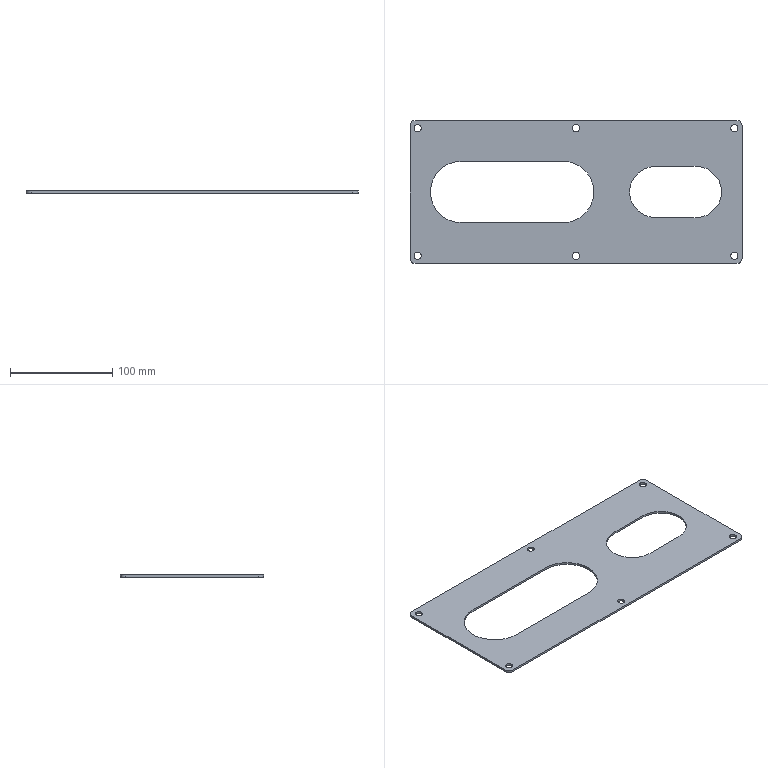Part | SolidWorks | features BaseBody 1 | 1 solid | 32 faces | box 325 x 140 x 2 mm | volume 64913 mm3 | cylinder 22 | plane 10 | commonest cylinder face diameters 7 x12 10 x4 50 x3 60 x3
STEP:
#1=CARTESIAN_POINT('',(-112.5,-30.,0.));
#2=VERTEX_POINT('',#1);
#3=CARTESIAN_POINT('',(-12.5,-30.,0.));
#4=VERTEX_POINT('',#3);
#5=CARTESIAN_POINT('',(-112.5,-30.,0.));
#6=DIRECTION('',(1.,0.,0.));
#7=VECTOR('',#6,1000.);
#8=LINE('',#5,#7);
#9=EDGE_CURVE('',#2,#4,#8,.T.);
#10=ORIENTED_EDGE('',*,*,#9,.T.);
#11=CARTESIAN_POINT('',(-12.5,-30.,-2.));
#12=VERTEX_POINT('',#11);
#13=CARTESIAN_POINT('',(-12.5,-30.,-2.));
#14=DIRECTION('',(0.,0.,1.));
#15=VECTOR('',#14,1000.);
#16=LINE('',#13,#15);
#17=EDGE_CURVE('',#12,#4,#16,.T.);
#18=ORIENTED_EDGE('',*,*,#17,.F.);
#19=CARTESIAN_POINT('',(-112.5,-30.,-2.));
#20=VERTEX_POINT('',#19);
#21=CARTESIAN_POINT('',(-112.5,-30.,-2.));
#22=DIRECTION('',(1.,0.,0.));
#23=VECTOR('',#22,1000.);
#24=LINE('',#21,#23);
#25=EDGE_CURVE('',#20,#12,#24,.T.);
#26=ORIENTED_EDGE('',*,*,#25,.F.);
#27=CARTESIAN_POINT('',(-112.5,-30.,-2.));
#28=DIRECTION('',(0.,0.,1.));
#29=VECTOR('',#28,1000.);
#30=LINE('',#27,#29);
#31=EDGE_CURVE('',#20,#2,#30,.T.);
#32=ORIENTED_EDGE('',*,*,#31,.T.);
#33=EDGE_LOOP('',(#10,#18,#26,#32));
#34=FACE_OUTER_BOUND('',#33,.T.);
#35=CARTESIAN_POINT('',(-112.5,-30.,-2.));
#36=DIRECTION('',(0.,-1.,0.));
#37=DIRECTION('',(-1.,0.,0.));
#38=AXIS2_PLACEMENT_3D('',#35,#36,#37);
#39=PLANE('',#38);
#40=ADVANCED_FACE('',(#34),#39,.F.);
#41=CARTESIAN_POINT('',(17.5,0.,-2.));
#42=VERTEX_POINT('',#41);
#43=CARTESIAN_POINT('',(17.5,0.,0.));
#44=VERTEX_POINT('',#43);
#45=CARTESIAN_POINT('',(17.5,0.,-2.));
#46=DIRECTION('',(0.,0.,1.));
#47=VECTOR('',#46,1000.);
#48=LINE('',#45,#47);
#49=EDGE_CURVE('',#42,#44,#48,.T.);
#50=ORIENTED_EDGE('',*,*,#49,.F.);
#51=CARTESIAN_POINT('',(-12.5,0.,-2.));
#52=DIRECTION('',(0.,0.,1.));
#53=DIRECTION('',(1.,0.,0.));
#54=AXIS2_PLACEMENT_3D('',#51,#52,#53);
#55=CIRCLE('',#54,30.);
#56=EDGE_CURVE('',#12,#42,#55,.T.);
#57=ORIENTED_EDGE('',*,*,#56,.F.);
#58=ORIENTED_EDGE('',*,*,#17,.T.);
#59=CARTESIAN_POINT('',(-12.5,0.,0.));
#60=DIRECTION('',(0.,0.,1.));
#61=DIRECTION('',(1.,0.,0.));
#62=AXIS2_PLACEMENT_3D('',#59,#60,#61);
#63=CIRCLE('',#62,30.);
#64=EDGE_CURVE('',#4,#44,#63,.T.);
#65=ORIENTED_EDGE('',*,*,#64,.T.);
#66=EDGE_LOOP('',(#50,#57,#58,#65));
#67=FACE_OUTER_BOUND('',#66,.T.);
#68=CARTESIAN_POINT('',(-12.5,0.,-2.));
#69=DIRECTION('',(0.,0.,1.));
#70=DIRECTION('',(1.,0.,0.));
#71=AXIS2_PLACEMENT_3D('',#68,#69,#70);
#72=CYLINDRICAL_SURFACE('',#71,30.);
#73=ADVANCED_FACE('',(#67),#72,.F.);
#74=CARTESIAN_POINT('',(-12.5,30.,0.));
#75=VERTEX_POINT('',#74);
#76=CARTESIAN_POINT('',(-112.5,30.,0.));
#77=VERTEX_POINT('',#76);
#78=CARTESIAN_POINT('',(-112.5,30.,0.));
#79=DIRECTION('',(-1.,0.,0.));
#80=VECTOR('',#79,1000.);
#81=LINE('',#78,#80);
#82=EDGE_CURVE('',#75,#77,#81,.T.);
#83=ORIENTED_EDGE('',*,*,#82,.T.);
#84=CARTESIAN_POINT('',(-112.5,30.,-2.));
#85=VERTEX_POINT('',#84);
#86=CARTESIAN_POINT('',(-112.5,30.,-2.));
#87=DIRECTION('',(0.,0.,1.));
#88=VECTOR('',#87,1000.);
#89=LINE('',#86,#88);
#90=EDGE_CURVE('',#85,#77,#89,.T.);
#91=ORIENTED_EDGE('',*,*,#90,.F.);
#92=CARTESIAN_POINT('',(-12.5,30.,-2.));
#93=VERTEX_POINT('',#92);
#94=CARTESIAN_POINT('',(-112.5,30.,-2.));
#95=DIRECTION('',(-1.,0.,0.));
#96=VECTOR('',#95,1000.);
#97=LINE('',#94,#96);
#98=EDGE_CURVE('',#93,#85,#97,.T.);
#99=ORIENTED_EDGE('',*,*,#98,.F.);
#100=CARTESIAN_POINT('',(-12.5,30.,-2.));
#101=DIRECTION('',(0.,0.,1.));
#102=VECTOR('',#101,1000.);
#103=LINE('',#100,#102);
#104=EDGE_CURVE('',#93,#75,#103,.T.);
#105=ORIENTED_EDGE('',*,*,#104,.T.);
#106=EDGE_LOOP('',(#83,#91,#99,#105));
#107=FACE_OUTER_BOUND('',#106,.T.);
#108=CARTESIAN_POINT('',(-112.5,30.,-2.));
#109=DIRECTION('',(0.,1.,0.));
#110=DIRECTION('',(1.,0.,0.));
#111=AXIS2_PLACEMENT_3D('',#108,#109,#110);
#112=PLANE('',#111);
#113=ADVANCED_FACE('',(#107),#112,.F.);
#114=CARTESIAN_POINT('',(-112.5,0.,0.));
#115=DIRECTION('',(0.,0.,1.));
#116=DIRECTION('',(1.,0.,0.));
#117=AXIS2_PLACEMENT_3D('',#114,#115,#116);
#118=CIRCLE('',#117,30.);
#119=EDGE_CURVE('',#77,#2,#118,.T.);
#120=ORIENTED_EDGE('',*,*,#119,.T.);
#121=ORIENTED_EDGE('',*,*,#31,.F.);
#122=CARTESIAN_POINT('',(-112.5,0.,-2.));
#123=DIRECTION('',(0.,0.,1.));
#124=DIRECTION('',(1.,0.,0.));
#125=AXIS2_PLACEMENT_3D('',#122,#123,#124);
#126=CIRCLE('',#125,30.);
#127=EDGE_CURVE('',#85,#20,#126,.T.);
#128=ORIENTED_EDGE('',*,*,#127,.F.);
#129=ORIENTED_EDGE('',*,*,#90,.T.);
#130=EDGE_LOOP('',(#120,#121,#128,#129));
#131=FACE_OUTER_BOUND('',#130,.T.);
#132=CARTESIAN_POINT('',(-112.5,0.,-2.));
#133=DIRECTION('',(0.,0.,1.));
#134=DIRECTION('',(1.,0.,0.));
#135=AXIS2_PLACEMENT_3D('',#132,#133,#134);
#136=CYLINDRICAL_SURFACE('',#135,30.);
#137=ADVANCED_FACE('',(#131),#136,.F.);
#138=CARTESIAN_POINT('',(77.5,-25.,0.));
#139=VERTEX_POINT('',#138);
#140=CARTESIAN_POINT('',(117.5,-25.,0.));
#141=VERTEX_POINT('',#140);
#142=CARTESIAN_POINT('',(77.5,-25.,0.));
#143=DIRECTION('',(1.,0.,0.));
#144=VECTOR('',#143,1000.);
#145=LINE('',#142,#144);
#146=EDGE_CURVE('',#139,#141,#145,.T.);
#147=ORIENTED_EDGE('',*,*,#146,.T.);
#148=CARTESIAN_POINT('',(117.5,-25.,-2.));
#149=VERTEX_POINT('',#148);
#150=CARTESIAN_POINT('',(117.5,-25.,-2.));
#151=DIRECTION('',(0.,0.,1.));
#152=VECTOR('',#151,1000.);
#153=LINE('',#150,#152);
#154=EDGE_CURVE('',#149,#141,#153,.T.);
#155=ORIENTED_EDGE('',*,*,#154,.F.);
#156=CARTESIAN_POINT('',(77.5,-25.,-2.));
#157=VERTEX_POINT('',#156);
#158=CARTESIAN_POINT('',(77.5,-25.,-2.));
#159=DIRECTION('',(1.,0.,0.));
#160=VECTOR('',#159,1000.);
#161=LINE('',#158,#160);
#162=EDGE_CURVE('',#157,#149,#161,.T.);
#163=ORIENTED_EDGE('',*,*,#162,.F.);
#164=CARTESIAN_POINT('',(77.5,-25.,-2.));
#165=DIRECTION('',(0.,0.,1.));
#166=VECTOR('',#165,1000.);
#167=LINE('',#164,#166);
#168=EDGE_CURVE('',#157,#139,#167,.T.);
#169=ORIENTED_EDGE('',*,*,#168,.T.);
#170=EDGE_LOOP('',(#147,#155,#163,#169));
#171=FACE_OUTER_BOUND('',#170,.T.);
#172=CARTESIAN_POINT('',(77.5,-25.,-2.));
#173=DIRECTION('',(0.,-1.,0.));
#174=DIRECTION('',(0.,0.,-1.));
#175=AXIS2_PLACEMENT_3D('',#172,#173,#174);
#176=PLANE('',#175);
#177=ADVANCED_FACE('',(#171),#176,.F.);
#178=CARTESIAN_POINT('',(142.5,0.,-2.));
#179=VERTEX_POINT('',#178);
#180=CARTESIAN_POINT('',(142.5,0.,0.));
#181=VERTEX_POINT('',#180);
#182=CARTESIAN_POINT('',(142.5,0.,-2.));
#183=DIRECTION('',(0.,0.,1.));
#184=VECTOR('',#183,1000.);
#185=LINE('',#182,#184);
#186=EDGE_CURVE('',#179,#181,#185,.T.);
#187=ORIENTED_EDGE('',*,*,#186,.F.);
#188=CARTESIAN_POINT('',(117.5,0.,-2.));
#189=DIRECTION('',(0.,0.,1.));
#190=DIRECTION('',(1.,0.,0.));
#191=AXIS2_PLACEMENT_3D('',#188,#189,#190);
#192=CIRCLE('',#191,25.);
#193=EDGE_CURVE('',#149,#179,#192,.T.);
#194=ORIENTED_EDGE('',*,*,#193,.F.);
#195=ORIENTED_EDGE('',*,*,#154,.T.);
#196=CARTESIAN_POINT('',(117.5,0.,0.));
#197=DIRECTION('',(0.,0.,1.));
#198=DIRECTION('',(1.,0.,0.));
#199=AXIS2_PLACEMENT_3D('',#196,#197,#198);
#200=CIRCLE('',#199,25.);
#201=EDGE_CURVE('',#141,#181,#200,.T.);
#202=ORIENTED_EDGE('',*,*,#201,.T.);
#203=EDGE_LOOP('',(#187,#194,#195,#202));
#204=FACE_OUTER_BOUND('',#203,.T.);
#205=CARTESIAN_POINT('',(117.5,0.,-2.));
#206=DIRECTION('',(0.,0.,1.));
#207=DIRECTION('',(1.,0.,0.));
#208=AXIS2_PLACEMENT_3D('',#205,#206,#207);
#209=CYLINDRICAL_SURFACE('',#208,25.);
#210=ADVANCED_FACE('',(#204),#209,.F.);
#211=CARTESIAN_POINT('',(117.5,25.,0.));
#212=VERTEX_POINT('',#211);
#213=CARTESIAN_POINT('',(77.5,25.,0.));
#214=VERTEX_POINT('',#213);
#215=CARTESIAN_POINT('',(77.5,25.,0.));
#216=DIRECTION('',(-1.,0.,0.));
#217=VECTOR('',#216,1000.);
#218=LINE('',#215,#217);
#219=EDGE_CURVE('',#212,#214,#218,.T.);
#220=ORIENTED_EDGE('',*,*,#219,.T.);
#221=CARTESIAN_POINT('',(77.5,25.,-2.));
#222=VERTEX_POINT('',#221);
#223=CARTESIAN_POINT('',(77.5,25.,-2.));
#224=DIRECTION('',(0.,0.,1.));
#225=VECTOR('',#224,1000.);
#226=LINE('',#223,#225);
#227=EDGE_CURVE('',#222,#214,#226,.T.);
#228=ORIENTED_EDGE('',*,*,#227,.F.);
#229=CARTESIAN_POINT('',(117.5,25.,-2.));
#230=VERTEX_POINT('',#229);
#231=CARTESIAN_POINT('',(77.5,25.,-2.));
#232=DIRECTION('',(-1.,0.,0.));
#233=VECTOR('',#232,1000.);
#234=LINE('',#231,#233);
#235=EDGE_CURVE('',#230,#222,#234,.T.);
#236=ORIENTED_EDGE('',*,*,#235,.F.);
#237=CARTESIAN_POINT('',(117.5,25.,-2.));
#238=DIRECTION('',(0.,0.,1.));
#239=VECTOR('',#238,1000.);
#240=LINE('',#237,#239);
#241=EDGE_CURVE('',#230,#212,#240,.T.);
#242=ORIENTED_EDGE('',*,*,#241,.T.);
#243=EDGE_LOOP('',(#220,#228,#236,#242));
#244=FACE_OUTER_BOUND('',#243,.T.);
#245=CARTESIAN_POINT('',(77.5,25.,-2.));
#246=DIRECTION('',(0.,1.,0.));
#247=DIRECTION('',(1.,0.,0.));
#248=AXIS2_PLACEMENT_3D('',#245,#246,#247);
#249=PLANE('',#248);
#250=ADVANCED_FACE('',(#244),#249,.F.);
#251=CARTESIAN_POINT('',(77.5,0.,0.));
#252=DIRECTION('',(0.,0.,1.));
#253=DIRECTION('',(1.,0.,0.));
#254=AXIS2_PLACEMENT_3D('',#251,#252,#253);
#255=CIRCLE('',#254,25.);
#256=EDGE_CURVE('',#214,#139,#255,.T.);
#257=ORIENTED_EDGE('',*,*,#256,.T.);
#258=ORIENTED_EDGE('',*,*,#168,.F.);
#259=CARTESIAN_POINT('',(77.5,0.,-2.));
#260=DIRECTION('',(0.,0.,1.));
#261=DIRECTION('',(1.,0.,0.));
#262=AXIS2_PLACEMENT_3D('',#259,#260,#261);
#263=CIRCLE('',#262,25.);
#264=EDGE_CURVE('',#222,#157,#263,.T.);
#265=ORIENTED_EDGE('',*,*,#264,.F.);
#266=ORIENTED_EDGE('',*,*,#227,.T.);
#267=EDGE_LOOP('',(#257,#258,#265,#266));
#268=FACE_OUTER_BOUND('',#267,.T.);
#269=CARTESIAN_POINT('',(77.5,0.,-2.));
#270=DIRECTION('',(0.,0.,1.));
#271=DIRECTION('',(1.,0.,0.));
#272=AXIS2_PLACEMENT_3D('',#269,#270,#271);
#273=CYLINDRICAL_SURFACE('',#272,25.);
#274=ADVANCED_FACE('',(#268),#273,.F.);
#275=CARTESIAN_POINT('',(-158.5,-62.5,-2.));
#276=VERTEX_POINT('',#275);
#277=CARTESIAN_POINT('',(-158.5,-62.5,0.));
#278=VERTEX_POINT('',#277);
#279=CARTESIAN_POINT('',(-158.5,-62.5,-2.));
#280=DIRECTION('',(0.,0.,1.));
#281=VECTOR('',#280,1000.);
#282=LINE('',#279,#281);
#283=EDGE_CURVE('',#276,#278,#282,.T.);
#284=ORIENTED_EDGE('',*,*,#283,.F.);
#285=CARTESIAN_POINT('',(-151.5,-62.5,-2.));
#286=VERTEX_POINT('',#285);
#287=CARTESIAN_POINT('',(-155.,-62.5,-2.));
#288=DIRECTION('',(0.,0.,1.));
#289=DIRECTION('',(-1.,0.,0.));
#290=AXIS2_PLACEMENT_3D('',#287,#288,#289);
#291=CIRCLE('',#290,3.5);
#292=EDGE_CURVE('',#286,#276,#291,.T.);
#293=ORIENTED_EDGE('',*,*,#292,.F.);
#294=CARTESIAN_POINT('',(-151.5,-62.5,0.));
#295=VERTEX_POINT('',#294);
#296=CARTESIAN_POINT('',(-151.5,-62.5,-2.));
#297=DIRECTION('',(0.,0.,1.));
#298=VECTOR('',#297,1000.);
#299=LINE('',#296,#298);
#300=EDGE_CURVE('',#286,#295,#299,.T.);
#301=ORIENTED_EDGE('',*,*,#300,.T.);
#302=CARTESIAN_POINT('',(-155.,-62.5,0.));
#303=DIRECTION('',(0.,0.,1.));
#304=DIRECTION('',(-1.,0.,0.));
#305=AXIS2_PLACEMENT_3D('',#302,#303,#304);
#306=CIRCLE('',#305,3.5);
#307=EDGE_CURVE('',#295,#278,#306,.T.);
#308=ORIENTED_EDGE('',*,*,#307,.T.);
#309=EDGE_LOOP('',(#284,#293,#301,#308));
#310=FACE_OUTER_BOUND('',#309,.T.);
#311=CARTESIAN_POINT('',(-155.,-62.5,-2.));
#312=DIRECTION('',(0.,0.,1.));
#313=DIRECTION('',(1.,0.,0.));
#314=AXIS2_PLACEMENT_3D('',#311,#312,#313);
#315=CYLINDRICAL_SURFACE('',#314,3.5);
#316=ADVANCED_FACE('',(#310),#315,.F.);
#317=CARTESIAN_POINT('',(-3.5,62.5,-2.));
#318=VERTEX_POINT('',#317);
#319=CARTESIAN_POINT('',(-3.5,62.5,0.));
#320=VERTEX_POINT('',#319);
#321=CARTESIAN_POINT('',(-3.5,62.5,-2.));
#322=DIRECTION('',(0.,0.,1.));
#323=VECTOR('',#322,1000.);
#324=LINE('',#321,#323);
#325=EDGE_CURVE('',#318,#320,#324,.T.);
#326=ORIENTED_EDGE('',*,*,#325,.F.);
#327=CARTESIAN_POINT('',(3.5,62.5,-2.));
#328=VERTEX_POINT('',#327);
#329=CARTESIAN_POINT('',(0.,62.5,-2.));
#330=DIRECTION('',(0.,0.,1.));
#331=DIRECTION('',(1.,0.,0.));
#332=AXIS2_PLACEMENT_3D('',#329,#330,#331);
#333=CIRCLE('',#332,3.5);
#334=EDGE_CURVE('',#328,#318,#333,.T.);
#335=ORIENTED_EDGE('',*,*,#334,.F.);
#336=CARTESIAN_POINT('',(3.5,62.5,0.));
#337=VERTEX_POINT('',#336);
#338=CARTESIAN_POINT('',(3.5,62.5,-2.));
#339=DIRECTION('',(0.,0.,1.));
#340=VECTOR('',#339,1000.);
#341=LINE('',#338,#340);
#342=EDGE_CURVE('',#328,#337,#341,.T.);
#343=ORIENTED_EDGE('',*,*,#342,.T.);
#344=CARTESIAN_POINT('',(0.,62.5,0.));
#345=DIRECTION('',(0.,0.,1.));
#346=DIRECTION('',(1.,0.,0.));
#347=AXIS2_PLACEMENT_3D('',#344,#345,#346);
#348=CIRCLE('',#347,3.5);
#349=EDGE_CURVE('',#337,#320,#348,.T.);
#350=ORIENTED_EDGE('',*,*,#349,.T.);
#351=EDGE_LOOP('',(#326,#335,#343,#350));
#352=FACE_OUTER_BOUND('',#351,.T.);
#353=CARTESIAN_POINT('',(0.,62.5,-2.));
#354=DIRECTION('',(0.,0.,1.));
#355=DIRECTION('',(1.,0.,0.));
#356=AXIS2_PLACEMENT_3D('',#353,#354,#355);
#357=CYLINDRICAL_SURFACE('',#356,3.5);
#358=ADVANCED_FACE('',(#352),#357,.F.);
#359=CARTESIAN_POINT('',(151.5,-62.5,-2.));
#360=VERTEX_POINT('',#359);
#361=CARTESIAN_POINT('',(151.5,-62.5,0.));
#362=VERTEX_POINT('',#361);
#363=CARTESIAN_POINT('',(151.5,-62.5,-2.));
#364=DIRECTION('',(0.,0.,1.));
#365=VECTOR('',#364,1000.);
#366=LINE('',#363,#365);
#367=EDGE_CURVE('',#360,#362,#366,.T.);
#368=ORIENTED_EDGE('',*,*,#367,.F.);
#369=CARTESIAN_POINT('',(158.5,-62.5,-2.));
#370=VERTEX_POINT('',#369);
#371=CARTESIAN_POINT('',(155.,-62.5,-2.));
#372=DIRECTION('',(0.,0.,1.));
#373=DIRECTION('',(1.,0.,0.));
#374=AXIS2_PLACEMENT_3D('',#371,#372,#373);
#375=CIRCLE('',#374,3.5);
#376=EDGE_CURVE('',#370,#360,#375,.T.);
#377=ORIENTED_EDGE('',*,*,#376,.F.);
#378=CARTESIAN_POINT('',(158.5,-62.5,0.));
#379=VERTEX_POINT('',#378);
#380=CARTESIAN_POINT('',(158.5,-62.5,-2.));
#381=DIRECTION('',(0.,0.,1.));
#382=VECTOR('',#381,1000.);
#383=LINE('',#380,#382);
#384=EDGE_CURVE('',#370,#379,#383,.T.);
#385=ORIENTED_EDGE('',*,*,#384,.T.);
#386=CARTESIAN_POINT('',(155.,-62.5,0.));
#387=DIRECTION('',(0.,0.,1.));
#388=DIRECTION('',(1.,0.,0.));
#389=AXIS2_PLACEMENT_3D('',#386,#387,#388);
#390=CIRCLE('',#389,3.5);
#391=EDGE_CURVE('',#379,#362,#390,.T.);
#392=ORIENTED_EDGE('',*,*,#391,.T.);
#393=EDGE_LOOP('',(#368,#377,#385,#392));
#394=FACE_OUTER_BOUND('',#393,.T.);
#395=CARTESIAN_POINT('',(155.,-62.5,-2.));
#396=DIRECTION('',(0.,0.,1.));
#397=DIRECTION('',(1.,0.,0.));
#398=AXIS2_PLACEMENT_3D('',#395,#396,#397);
#399=CYLINDRICAL_SURFACE('',#398,3.5);
#400=ADVANCED_FACE('',(#394),#399,.F.);
#401=CARTESIAN_POINT('',(151.5,62.5,-2.));
#402=VERTEX_POINT('',#401);
#403=CARTESIAN_POINT('',(151.5,62.5,0.));
#404=VERTEX_POINT('',#403);
#405=CARTESIAN_POINT('',(151.5,62.5,-2.));
#406=DIRECTION('',(0.,0.,1.));
#407=VECTOR('',#406,1000.);
#408=LINE('',#405,#407);
#409=EDGE_CURVE('',#402,#404,#408,.T.);
#410=ORIENTED_EDGE('',*,*,#409,.F.);
#411=CARTESIAN_POINT('',(158.5,62.5,-2.));
#412=VERTEX_POINT('',#411);
#413=CARTESIAN_POINT('',(155.,62.5,-2.));
#414=DIRECTION('',(0.,0.,1.));
#415=DIRECTION('',(-1.,0.,0.));
#416=AXIS2_PLACEMENT_3D('',#413,#414,#415);
#417=CIRCLE('',#416,3.5);
#418=EDGE_CURVE('',#412,#402,#417,.T.);
#419=ORIENTED_EDGE('',*,*,#418,.F.);
#420=CARTESIAN_POINT('',(158.5,62.5,0.));
#421=VERTEX_POINT('',#420);
#422=CARTESIAN_POINT('',(158.5,62.5,-2.));
#423=DIRECTION('',(0.,0.,1.));
#424=VECTOR('',#423,1000.);
#425=LINE('',#422,#424);
#426=EDGE_CURVE('',#412,#421,#425,.T.);
#427=ORIENTED_EDGE('',*,*,#426,.T.);
#428=CARTESIAN_POINT('',(155.,62.5,0.));
#429=DIRECTION('',(0.,0.,1.));
#430=DIRECTION('',(-1.,0.,0.));
#431=AXIS2_PLACEMENT_3D('',#428,#429,#430);
#432=CIRCLE('',#431,3.5);
#433=EDGE_CURVE('',#421,#404,#432,.T.);
#434=ORIENTED_EDGE('',*,*,#433,.T.);
#435=EDGE_LOOP('',(#410,#419,#427,#434));
#436=FACE_OUTER_BOUND('',#435,.T.);
#437=CARTESIAN_POINT('',(155.,62.5,-2.));
#438=DIRECTION('',(0.,0.,1.));
#439=DIRECTION('',(1.,0.,0.));
#440=AXIS2_PLACEMENT_3D('',#437,#438,#439);
#441=CYLINDRICAL_SURFACE('',#440,3.5);
#442=ADVANCED_FACE('',(#436),#441,.F.);
#443=CARTESIAN_POINT('',(-3.5,-62.5,-2.));
#444=VERTEX_POINT('',#443);
#445=CARTESIAN_POINT('',(-3.5,-62.5,0.));
#446=VERTEX_POINT('',#445);
#447=CARTESIAN_POINT('',(-3.5,-62.5,-2.));
#448=DIRECTION('',(0.,0.,1.));
#449=VECTOR('',#448,1000.);
#450=LINE('',#447,#449);
#451=EDGE_CURVE('',#444,#446,#450,.T.);
#452=ORIENTED_EDGE('',*,*,#451,.F.);
#453=CARTESIAN_POINT('',(3.5,-62.5,-2.));
#454=VERTEX_POINT('',#453);
#455=CARTESIAN_POINT('',(0.,-62.5,-2.));
#456=DIRECTION('',(0.,0.,1.));
#457=DIRECTION('',(-1.,0.,0.));
#458=AXIS2_PLACEMENT_3D('',#455,#456,#457);
#459=CIRCLE('',#458,3.5);
#460=EDGE_CURVE('',#454,#444,#459,.T.);
#461=ORIENTED_EDGE('',*,*,#460,.F.);
#462=CARTESIAN_POINT('',(3.5,-62.5,0.));
#463=VERTEX_POINT('',#462);
#464=CARTESIAN_POINT('',(3.5,-62.5,-2.));
#465=DIRECTION('',(0.,0.,1.));
#466=VECTOR('',#465,1000.);
#467=LINE('',#464,#466);
#468=EDGE_CURVE('',#454,#463,#467,.T.);
#469=ORIENTED_EDGE('',*,*,#468,.T.);
#470=CARTESIAN_POINT('',(0.,-62.5,0.));
#471=DIRECTION('',(0.,0.,1.));
#472=DIRECTION('',(-1.,0.,0.));
#473=AXIS2_PLACEMENT_3D('',#470,#471,#472);
#474=CIRCLE('',#473,3.5);
#475=EDGE_CURVE('',#463,#446,#474,.T.);
#476=ORIENTED_EDGE('',*,*,#475,.T.);
#477=EDGE_LOOP('',(#452,#461,#469,#476));
#478=FACE_OUTER_BOUND('',#477,.T.);
#479=CARTESIAN_POINT('',(0.,-62.5,-2.));
#480=DIRECTION('',(0.,0.,1.));
#481=DIRECTION('',(1.,0.,0.));
#482=AXIS2_PLACEMENT_3D('',#479,#480,#481);
#483=CYLINDRICAL_SURFACE('',#482,3.5);
#484=ADVANCED_FACE('',(#478),#483,.F.);
#485=CARTESIAN_POINT('',(-158.5,62.5,-2.));
#486=VERTEX_POINT('',#485);
#487=CARTESIAN_POINT('',(-158.5,62.5,0.));
#488=VERTEX_POINT('',#487);
#489=CARTESIAN_POINT('',(-158.5,62.5,-2.));
#490=DIRECTION('',(0.,0.,1.));
#491=VECTOR('',#490,1000.);
#492=LINE('',#489,#491);
#493=EDGE_CURVE('',#486,#488,#492,.T.);
#494=ORIENTED_EDGE('',*,*,#493,.F.);
#495=CARTESIAN_POINT('',(-151.5,62.5,-2.));
#496=VERTEX_POINT('',#495);
#497=CARTESIAN_POINT('',(-155.,62.5,-2.));
#498=DIRECTION('',(0.,0.,1.));
#499=DIRECTION('',(1.,0.,0.));
#500=AXIS2_PLACEMENT_3D('',#497,#498,#499);
#501=CIRCLE('',#500,3.5);
#502=EDGE_CURVE('',#496,#486,#501,.T.);
#503=ORIENTED_EDGE('',*,*,#502,.F.);
#504=CARTESIAN_POINT('',(-151.5,62.5,0.));
#505=VERTEX_POINT('',#504);
#506=CARTESIAN_POINT('',(-151.5,62.5,-2.));
#507=DIRECTION('',(0.,0.,1.));
#508=VECTOR('',#507,1000.);
#509=LINE('',#506,#508);
#510=EDGE_CURVE('',#496,#505,#509,.T.);
#511=ORIENTED_EDGE('',*,*,#510,.T.);
#512=CARTESIAN_POINT('',(-155.,62.5,0.));
#513=DIRECTION('',(0.,0.,1.));
#514=DIRECTION('',(1.,0.,0.));
#515=AXIS2_PLACEMENT_3D('',#512,#513,#514);
#516=CIRCLE('',#515,3.5);
#517=EDGE_CURVE('',#505,#488,#516,.T.);
#518=ORIENTED_EDGE('',*,*,#517,.T.);
#519=EDGE_LOOP('',(#494,#503,#511,#518));
#520=FACE_OUTER_BOUND('',#519,.T.);
#521=CARTESIAN_POINT('',(-155.,62.5,-2.));
#522=DIRECTION('',(0.,0.,1.));
#523=DIRECTION('',(1.,0.,0.));
#524=AXIS2_PLACEMENT_3D('',#521,#522,#523);
#525=CYLINDRICAL_SURFACE('',#524,3.5);
#526=ADVANCED_FACE('',(#520),#525,.F.);
#527=CARTESIAN_POINT('',(-162.5,65.,-2.));
#528=VERTEX_POINT('',#527);
#529=CARTESIAN_POINT('',(-157.5,70.,-2.));
#530=VERTEX_POINT('',#529);
#531=CARTESIAN_POINT('',(-157.5,65.,-2.));
#532=DIRECTION('',(0.,0.,-1.));
#533=DIRECTION('',(-1.,0.,0.));
#534=AXIS2_PLACEMENT_3D('',#531,#532,#533);
#535=CIRCLE('',#534,5.);
#536=EDGE_CURVE('',#528,#530,#535,.T.);
#537=ORIENTED_EDGE('',*,*,#536,.F.);
#538=CARTESIAN_POINT('',(-162.5,65.,0.));
#539=VERTEX_POINT('',#538);
#540=CARTESIAN_POINT('',(-162.5,65.,-2.));
#541=DIRECTION('',(0.,0.,-1.));
#542=VECTOR('',#541,1000.);
#543=LINE('',#540,#542);
#544=EDGE_CURVE('',#539,#528,#543,.T.);
#545=ORIENTED_EDGE('',*,*,#544,.F.);
#546=CARTESIAN_POINT('',(-157.5,70.,0.));
#547=VERTEX_POINT('',#546);
#548=CARTESIAN_POINT('',(-157.5,65.,0.));
#549=DIRECTION('',(0.,0.,1.));
#550=DIRECTION('',(-1.,0.,0.));
#551=AXIS2_PLACEMENT_3D('',#548,#549,#550);
#552=CIRCLE('',#551,5.);
#553=EDGE_CURVE('',#547,#539,#552,.T.);
#554=ORIENTED_EDGE('',*,*,#553,.F.);
#555=CARTESIAN_POINT('',(-157.5,70.,-2.));
#556=DIRECTION('',(0.,0.,1.));
#557=VECTOR('',#556,1000.);
#558=LINE('',#555,#557);
#559=EDGE_CURVE('',#530,#547,#558,.T.);
#560=ORIENTED_EDGE('',*,*,#559,.F.);
#561=EDGE_LOOP('',(#537,#545,#554,#560));
#562=FACE_OUTER_BOUND('',#561,.T.);
#563=CARTESIAN_POINT('',(-157.5,65.,-2.));
#564=DIRECTION('',(0.,0.,1.));
#565=DIRECTION('',(1.,0.,0.));
#566=AXIS2_PLACEMENT_3D('',#563,#564,#565);
#567=CYLINDRICAL_SURFACE('',#566,5.);
#568=ADVANCED_FACE('',(#562),#567,.T.);
#569=CARTESIAN_POINT('',(-157.5,-70.,-2.));
#570=VERTEX_POINT('',#569);
#571=CARTESIAN_POINT('',(-162.5,-65.,-2.));
#572=VERTEX_POINT('',#571);
#573=CARTESIAN_POINT('',(-157.5,-65.,-2.));
#574=DIRECTION('',(0.,0.,-1.));
#575=DIRECTION('',(-1.,0.,0.));
#576=AXIS2_PLACEMENT_3D('',#573,#574,#575);
#577=CIRCLE('',#576,5.);
#578=EDGE_CURVE('',#570,#572,#577,.T.);
#579=ORIENTED_EDGE('',*,*,#578,.F.);
#580=CARTESIAN_POINT('',(-157.5,-70.,0.));
#581=VERTEX_POINT('',#580);
#582=CARTESIAN_POINT('',(-157.5,-70.,-2.));
#583=DIRECTION('',(0.,0.,-1.));
#584=VECTOR('',#583,1000.);
#585=LINE('',#582,#584);
#586=EDGE_CURVE('',#581,#570,#585,.T.);
#587=ORIENTED_EDGE('',*,*,#586,.F.);
#588=CARTESIAN_POINT('',(-162.5,-65.,0.));
#589=VERTEX_POINT('',#588);
#590=CARTESIAN_POINT('',(-157.5,-65.,0.));
#591=DIRECTION('',(0.,0.,1.));
#592=DIRECTION('',(-1.,0.,0.));
#593=AXIS2_PLACEMENT_3D('',#590,#591,#592);
#594=CIRCLE('',#593,5.);
#595=EDGE_CURVE('',#589,#581,#594,.T.);
#596=ORIENTED_EDGE('',*,*,#595,.F.);
#597=CARTESIAN_POINT('',(-162.5,-65.,-2.));
#598=DIRECTION('',(0.,0.,1.));
#599=VECTOR('',#598,1000.);
#600=LINE('',#597,#599);
#601=EDGE_CURVE('',#572,#589,#600,.T.);
#602=ORIENTED_EDGE('',*,*,#601,.F.);
#603=EDGE_LOOP('',(#579,#587,#596,#602));
#604=FACE_OUTER_BOUND('',#603,.T.);
#605=CARTESIAN_POINT('',(-157.5,-65.,-2.));
#606=DIRECTION('',(0.,0.,1.));
#607=DIRECTION('',(1.,0.,0.));
#608=AXIS2_PLACEMENT_3D('',#605,#606,#607);
#609=CYLINDRICAL_SURFACE('',#608,5.);
#610=ADVANCED_FACE('',(#604),#609,.T.);
#611=CARTESIAN_POINT('',(162.5,-65.,-2.));
#612=VERTEX_POINT('',#611);
#613=CARTESIAN_POINT('',(157.5,-70.,-2.));
#614=VERTEX_POINT('',#613);
#615=CARTESIAN_POINT('',(157.5,-65.,-2.));
#616=DIRECTION('',(0.,0.,-1.));
#617=DIRECTION('',(-1.,0.,0.));
#618=AXIS2_PLACEMENT_3D('',#615,#616,#617);
#619=CIRCLE('',#618,5.);
#620=EDGE_CURVE('',#612,#614,#619,.T.);
#621=ORIENTED_EDGE('',*,*,#620,.F.);
#622=CARTESIAN_POINT('',(162.5,-65.,0.));
#623=VERTEX_POINT('',#622);
#624=CARTESIAN_POINT('',(162.5,-65.,-2.));
#625=DIRECTION('',(0.,0.,-1.));
#626=VECTOR('',#625,1000.);
#627=LINE('',#624,#626);
#628=EDGE_CURVE('',#623,#612,#627,.T.);
#629=ORIENTED_EDGE('',*,*,#628,.F.);
#630=CARTESIAN_POINT('',(157.5,-70.,0.));
#631=VERTEX_POINT('',#630);
#632=CARTESIAN_POINT('',(157.5,-65.,0.));
#633=DIRECTION('',(0.,0.,1.));
#634=DIRECTION('',(-1.,0.,0.));
#635=AXIS2_PLACEMENT_3D('',#632,#633,#634);
#636=CIRCLE('',#635,5.);
#637=EDGE_CURVE('',#631,#623,#636,.T.);
#638=ORIENTED_EDGE('',*,*,#637,.F.);
#639=CARTESIAN_POINT('',(157.5,-70.,-2.));
#640=DIRECTION('',(0.,0.,1.));
#641=VECTOR('',#640,1000.);
#642=LINE('',#639,#641);
#643=EDGE_CURVE('',#614,#631,#642,.T.);
#644=ORIENTED_EDGE('',*,*,#643,.F.);
#645=EDGE_LOOP('',(#621,#629,#638,#644));
#646=FACE_OUTER_BOUND('',#645,.T.);
#647=CARTESIAN_POINT('',(157.5,-65.,-2.));
#648=DIRECTION('',(0.,0.,1.));
#649=DIRECTION('',(1.,0.,0.));
#650=AXIS2_PLACEMENT_3D('',#647,#648,#649);
#651=CYLINDRICAL_SURFACE('',#650,5.);
#652=ADVANCED_FACE('',(#646),#651,.T.);
#653=CARTESIAN_POINT('',(157.5,70.,-2.));
#654=VERTEX_POINT('',#653);
#655=CARTESIAN_POINT('',(162.5,65.,-2.));
#656=VERTEX_POINT('',#655);
#657=CARTESIAN_POINT('',(157.5,65.,-2.));
#658=DIRECTION('',(0.,0.,-1.));
#659=DIRECTION('',(-1.,0.,0.));
#660=AXIS2_PLACEMENT_3D('',#657,#658,#659);
#661=CIRCLE('',#660,5.);
#662=EDGE_CURVE('',#654,#656,#661,.T.);
#663=ORIENTED_EDGE('',*,*,#662,.F.);
#664=CARTESIAN_POINT('',(157.5,70.,0.));
#665=VERTEX_POINT('',#664);
#666=CARTESIAN_POINT('',(157.5,70.,-2.));
#667=DIRECTION('',(0.,0.,-1.));
#668=VECTOR('',#667,1000.);
#669=LINE('',#666,#668);
#670=EDGE_CURVE('',#665,#654,#669,.T.);
#671=ORIENTED_EDGE('',*,*,#670,.F.);
#672=CARTESIAN_POINT('',(162.5,65.,0.));
#673=VERTEX_POINT('',#672);
#674=CARTESIAN_POINT('',(157.5,65.,0.));
#675=DIRECTION('',(0.,0.,1.));
#676=DIRECTION('',(-1.,0.,0.));
#677=AXIS2_PLACEMENT_3D('',#674,#675,#676);
#678=CIRCLE('',#677,5.);
#679=EDGE_CURVE('',#673,#665,#678,.T.);
#680=ORIENTED_EDGE('',*,*,#679,.F.);
#681=CARTESIAN_POINT('',(162.5,65.,-2.));
#682=DIRECTION('',(0.,0.,1.));
#683=VECTOR('',#682,1000.);
#684=LINE('',#681,#683);
#685=EDGE_CURVE('',#656,#673,#684,.T.);
#686=ORIENTED_EDGE('',*,*,#685,.F.);
#687=EDGE_LOOP('',(#663,#671,#680,#686));
#688=FACE_OUTER_BOUND('',#687,.T.);
#689=CARTESIAN_POINT('',(157.5,65.,-2.));
#690=DIRECTION('',(0.,0.,1.));
#691=DIRECTION('',(1.,0.,0.));
#692=AXIS2_PLACEMENT_3D('',#689,#690,#691);
#693=CYLINDRICAL_SURFACE('',#692,5.);
#694=ADVANCED_FACE('',(#688),#693,.T.);
#695=ORIENTED_EDGE('',*,*,#517,.F.);
#696=CARTESIAN_POINT('',(-155.,62.5,0.));
#697=DIRECTION('',(0.,0.,1.));
#698=DIRECTION('',(1.,0.,0.));
#699=AXIS2_PLACEMENT_3D('',#696,#697,#698);
#700=CIRCLE('',#699,3.5);
#701=EDGE_CURVE('',#488,#505,#700,.T.);
#702=ORIENTED_EDGE('',*,*,#701,.F.);
#703=EDGE_LOOP('',(#695,#702));
#704=FACE_BOUND('',#703,.T.);
#705=ORIENTED_EDGE('',*,*,#475,.F.);
#706=CARTESIAN_POINT('',(0.,-62.5,0.));
#707=DIRECTION('',(0.,0.,1.));
#708=DIRECTION('',(-1.,0.,0.));
#709=AXIS2_PLACEMENT_3D('',#706,#707,#708);
#710=CIRCLE('',#709,3.5);
#711=EDGE_CURVE('',#446,#463,#710,.T.);
#712=ORIENTED_EDGE('',*,*,#711,.F.);
#713=EDGE_LOOP('',(#705,#712));
#714=FACE_BOUND('',#713,.T.);
#715=ORIENTED_EDGE('',*,*,#433,.F.);
#716=CARTESIAN_POINT('',(155.,62.5,0.));
#717=DIRECTION('',(0.,0.,1.));
#718=DIRECTION('',(-1.,0.,0.));
#719=AXIS2_PLACEMENT_3D('',#716,#717,#718);
#720=CIRCLE('',#719,3.5);
#721=EDGE_CURVE('',#404,#421,#720,.T.);
#722=ORIENTED_EDGE('',*,*,#721,.F.);
#723=EDGE_LOOP('',(#715,#722));
#724=FACE_BOUND('',#723,.T.);
#725=ORIENTED_EDGE('',*,*,#391,.F.);
#726=CARTESIAN_POINT('',(155.,-62.5,0.));
#727=DIRECTION('',(0.,0.,1.));
#728=DIRECTION('',(1.,0.,0.));
#729=AXIS2_PLACEMENT_3D('',#726,#727,#728);
#730=CIRCLE('',#729,3.5);
#731=EDGE_CURVE('',#362,#379,#730,.T.);
#732=ORIENTED_EDGE('',*,*,#731,.F.);
#733=EDGE_LOOP('',(#725,#732));
#734=FACE_BOUND('',#733,.T.);
#735=ORIENTED_EDGE('',*,*,#349,.F.);
#736=CARTESIAN_POINT('',(0.,62.5,0.));
#737=DIRECTION('',(0.,0.,1.));
#738=DIRECTION('',(1.,0.,0.));
#739=AXIS2_PLACEMENT_3D('',#736,#737,#738);
#740=CIRCLE('',#739,3.5);
#741=EDGE_CURVE('',#320,#337,#740,.T.);
#742=ORIENTED_EDGE('',*,*,#741,.F.);
#743=EDGE_LOOP('',(#735,#742));
#744=FACE_BOUND('',#743,.T.);
#745=ORIENTED_EDGE('',*,*,#307,.F.);
#746=CARTESIAN_POINT('',(-155.,-62.5,0.));
#747=DIRECTION('',(0.,0.,1.));
#748=DIRECTION('',(-1.,0.,0.));
#749=AXIS2_PLACEMENT_3D('',#746,#747,#748);
#750=CIRCLE('',#749,3.5);
#751=EDGE_CURVE('',#278,#295,#750,.T.);
#752=ORIENTED_EDGE('',*,*,#751,.F.);
#753=EDGE_LOOP('',(#745,#752));
#754=FACE_BOUND('',#753,.T.);
#755=ORIENTED_EDGE('',*,*,#146,.F.);
#756=ORIENTED_EDGE('',*,*,#256,.F.);
#757=ORIENTED_EDGE('',*,*,#219,.F.);
#758=CARTESIAN_POINT('',(117.5,0.,0.));
#759=DIRECTION('',(0.,0.,1.));
#760=DIRECTION('',(1.,0.,0.));
#761=AXIS2_PLACEMENT_3D('',#758,#759,#760);
#762=CIRCLE('',#761,25.);
#763=EDGE_CURVE('',#181,#212,#762,.T.);
#764=ORIENTED_EDGE('',*,*,#763,.F.);
#765=ORIENTED_EDGE('',*,*,#201,.F.);
#766=EDGE_LOOP('',(#755,#756,#757,#764,#765));
#767=FACE_BOUND('',#766,.T.);
#768=ORIENTED_EDGE('',*,*,#9,.F.);
#769=ORIENTED_EDGE('',*,*,#119,.F.);
#770=ORIENTED_EDGE('',*,*,#82,.F.);
#771=CARTESIAN_POINT('',(-12.5,0.,0.));
#772=DIRECTION('',(0.,0.,1.));
#773=DIRECTION('',(1.,0.,0.));
#774=AXIS2_PLACEMENT_3D('',#771,#772,#773);
#775=CIRCLE('',#774,30.);
#776=EDGE_CURVE('',#44,#75,#775,.T.);
#777=ORIENTED_EDGE('',*,*,#776,.F.);
#778=ORIENTED_EDGE('',*,*,#64,.F.);
#779=EDGE_LOOP('',(#768,#769,#770,#777,#778));
#780=FACE_BOUND('',#779,.T.);
#781=CARTESIAN_POINT('',(162.5,70.,0.));
#782=DIRECTION('',(0.,1.,0.));
#783=VECTOR('',#782,1000.);
#784=LINE('',#781,#783);
#785=EDGE_CURVE('',#623,#673,#784,.T.);
#786=ORIENTED_EDGE('',*,*,#785,.T.);
#787=ORIENTED_EDGE('',*,*,#679,.T.);
#788=CARTESIAN_POINT('',(162.5,70.,0.));
#789=DIRECTION('',(-1.,0.,0.));
#790=VECTOR('',#789,1000.);
#791=LINE('',#788,#790);
#792=EDGE_CURVE('',#665,#547,#791,.T.);
#793=ORIENTED_EDGE('',*,*,#792,.T.);
#794=ORIENTED_EDGE('',*,*,#553,.T.);
#795=CARTESIAN_POINT('',(-162.5,70.,0.));
#796=DIRECTION('',(0.,-1.,0.));
#797=VECTOR('',#796,1000.);
#798=LINE('',#795,#797);
#799=EDGE_CURVE('',#539,#589,#798,.T.);
#800=ORIENTED_EDGE('',*,*,#799,.T.);
#801=ORIENTED_EDGE('',*,*,#595,.T.);
#802=CARTESIAN_POINT('',(162.5,-70.,0.));
#803=DIRECTION('',(1.,0.,0.));
#804=VECTOR('',#803,1000.);
#805=LINE('',#802,#804);
#806=EDGE_CURVE('',#581,#631,#805,.T.);
#807=ORIENTED_EDGE('',*,*,#806,.T.);
#808=ORIENTED_EDGE('',*,*,#637,.T.);
#809=EDGE_LOOP('',(#786,#787,#793,#794,#800,#801,#807,#808));
#810=FACE_OUTER_BOUND('',#809,.T.);
#811=CARTESIAN_POINT('',(0.,0.,0.));
#812=DIRECTION('',(0.,0.,-1.));
#813=DIRECTION('',(0.,-1.,0.));
#814=AXIS2_PLACEMENT_3D('',#811,#812,#813);
#815=PLANE('',#814);
#816=ADVANCED_FACE('',(#704,#714,#724,#734,#744,#754,#767,#780,#810),#815,.F.);
#817=ORIENTED_EDGE('',*,*,#502,.T.);
#818=CARTESIAN_POINT('',(-155.,62.5,-2.));
#819=DIRECTION('',(0.,0.,1.));
#820=DIRECTION('',(1.,0.,0.));
#821=AXIS2_PLACEMENT_3D('',#818,#819,#820);
#822=CIRCLE('',#821,3.5);
#823=EDGE_CURVE('',#486,#496,#822,.T.);
#824=ORIENTED_EDGE('',*,*,#823,.T.);
#825=EDGE_LOOP('',(#817,#824));
#826=FACE_BOUND('',#825,.T.);
#827=ORIENTED_EDGE('',*,*,#460,.T.);
#828=CARTESIAN_POINT('',(0.,-62.5,-2.));
#829=DIRECTION('',(0.,0.,1.));
#830=DIRECTION('',(-1.,0.,0.));
#831=AXIS2_PLACEMENT_3D('',#828,#829,#830);
#832=CIRCLE('',#831,3.5);
#833=EDGE_CURVE('',#444,#454,#832,.T.);
#834=ORIENTED_EDGE('',*,*,#833,.T.);
#835=EDGE_LOOP('',(#827,#834));
#836=FACE_BOUND('',#835,.T.);
#837=ORIENTED_EDGE('',*,*,#418,.T.);
#838=CARTESIAN_POINT('',(155.,62.5,-2.));
#839=DIRECTION('',(0.,0.,1.));
#840=DIRECTION('',(-1.,0.,0.));
#841=AXIS2_PLACEMENT_3D('',#838,#839,#840);
#842=CIRCLE('',#841,3.5);
#843=EDGE_CURVE('',#402,#412,#842,.T.);
#844=ORIENTED_EDGE('',*,*,#843,.T.);
#845=EDGE_LOOP('',(#837,#844));
#846=FACE_BOUND('',#845,.T.);
#847=ORIENTED_EDGE('',*,*,#376,.T.);
#848=CARTESIAN_POINT('',(155.,-62.5,-2.));
#849=DIRECTION('',(0.,0.,1.));
#850=DIRECTION('',(1.,0.,0.));
#851=AXIS2_PLACEMENT_3D('',#848,#849,#850);
#852=CIRCLE('',#851,3.5);
#853=EDGE_CURVE('',#360,#370,#852,.T.);
#854=ORIENTED_EDGE('',*,*,#853,.T.);
#855=EDGE_LOOP('',(#847,#854));
#856=FACE_BOUND('',#855,.T.);
#857=ORIENTED_EDGE('',*,*,#334,.T.);
#858=CARTESIAN_POINT('',(0.,62.5,-2.));
#859=DIRECTION('',(0.,0.,1.));
#860=DIRECTION('',(1.,0.,0.));
#861=AXIS2_PLACEMENT_3D('',#858,#859,#860);
#862=CIRCLE('',#861,3.5);
#863=EDGE_CURVE('',#318,#328,#862,.T.);
#864=ORIENTED_EDGE('',*,*,#863,.T.);
#865=EDGE_LOOP('',(#857,#864));
#866=FACE_BOUND('',#865,.T.);
#867=ORIENTED_EDGE('',*,*,#292,.T.);
#868=CARTESIAN_POINT('',(-155.,-62.5,-2.));
#869=DIRECTION('',(0.,0.,1.));
#870=DIRECTION('',(-1.,0.,0.));
#871=AXIS2_PLACEMENT_3D('',#868,#869,#870);
#872=CIRCLE('',#871,3.5);
#873=EDGE_CURVE('',#276,#286,#872,.T.);
#874=ORIENTED_EDGE('',*,*,#873,.T.);
#875=EDGE_LOOP('',(#867,#874));
#876=FACE_BOUND('',#875,.T.);
#877=ORIENTED_EDGE('',*,*,#264,.T.);
#878=ORIENTED_EDGE('',*,*,#162,.T.);
#879=ORIENTED_EDGE('',*,*,#193,.T.);
#880=CARTESIAN_POINT('',(117.5,0.,-2.));
#881=DIRECTION('',(0.,0.,1.));
#882=DIRECTION('',(1.,0.,0.));
#883=AXIS2_PLACEMENT_3D('',#880,#881,#882);
#884=CIRCLE('',#883,25.);
#885=EDGE_CURVE('',#179,#230,#884,.T.);
#886=ORIENTED_EDGE('',*,*,#885,.T.);
#887=ORIENTED_EDGE('',*,*,#235,.T.);
#888=EDGE_LOOP('',(#877,#878,#879,#886,#887));
#889=FACE_BOUND('',#888,.T.);
#890=ORIENTED_EDGE('',*,*,#127,.T.);
#891=ORIENTED_EDGE('',*,*,#25,.T.);
#892=ORIENTED_EDGE('',*,*,#56,.T.);
#893=CARTESIAN_POINT('',(-12.5,0.,-2.));
#894=DIRECTION('',(0.,0.,1.));
#895=DIRECTION('',(1.,0.,0.));
#896=AXIS2_PLACEMENT_3D('',#893,#894,#895);
#897=CIRCLE('',#896,30.);
#898=EDGE_CURVE('',#42,#93,#897,.T.);
#899=ORIENTED_EDGE('',*,*,#898,.T.);
#900=ORIENTED_EDGE('',*,*,#98,.T.);
#901=EDGE_LOOP('',(#890,#891,#892,#899,#900));
#902=FACE_BOUND('',#901,.T.);
#903=CARTESIAN_POINT('',(162.5,70.,-2.));
#904=DIRECTION('',(-1.,0.,0.));
#905=VECTOR('',#904,1000.);
#906=LINE('',#903,#905);
#907=EDGE_CURVE('',#654,#530,#906,.T.);
#908=ORIENTED_EDGE('',*,*,#907,.F.);
#909=ORIENTED_EDGE('',*,*,#662,.T.);
#910=CARTESIAN_POINT('',(162.5,70.,-2.));
#911=DIRECTION('',(0.,1.,0.));
#912=VECTOR('',#911,1000.);
#913=LINE('',#910,#912);
#914=EDGE_CURVE('',#612,#656,#913,.T.);
#915=ORIENTED_EDGE('',*,*,#914,.F.);
#916=ORIENTED_EDGE('',*,*,#620,.T.);
#917=CARTESIAN_POINT('',(162.5,-70.,-2.));
#918=DIRECTION('',(1.,0.,0.));
#919=VECTOR('',#918,1000.);
#920=LINE('',#917,#919);
#921=EDGE_CURVE('',#570,#614,#920,.T.);
#922=ORIENTED_EDGE('',*,*,#921,.F.);
#923=ORIENTED_EDGE('',*,*,#578,.T.);
#924=CARTESIAN_POINT('',(-162.5,70.,-2.));
#925=DIRECTION('',(0.,-1.,0.));
#926=VECTOR('',#925,1000.);
#927=LINE('',#924,#926);
#928=EDGE_CURVE('',#528,#572,#927,.T.);
#929=ORIENTED_EDGE('',*,*,#928,.F.);
#930=ORIENTED_EDGE('',*,*,#536,.T.);
#931=EDGE_LOOP('',(#908,#909,#915,#916,#922,#923,#929,#930));
#932=FACE_OUTER_BOUND('',#931,.T.);
#933=CARTESIAN_POINT('',(0.,0.,-2.));
#934=DIRECTION('',(0.,0.,-1.));
#935=DIRECTION('',(0.,-1.,0.));
#936=AXIS2_PLACEMENT_3D('',#933,#934,#935);
#937=PLANE('',#936);
#938=ADVANCED_FACE('',(#826,#836,#846,#856,#866,#876,#889,#902,#932),#937,.T.);
#939=ORIENTED_EDGE('',*,*,#921,.T.);
#940=ORIENTED_EDGE('',*,*,#643,.T.);
#941=ORIENTED_EDGE('',*,*,#806,.F.);
#942=ORIENTED_EDGE('',*,*,#586,.T.);
#943=EDGE_LOOP('',(#939,#940,#941,#942));
#944=FACE_OUTER_BOUND('',#943,.T.);
#945=CARTESIAN_POINT('',(162.5,-70.,-2.));
#946=DIRECTION('',(0.,-1.,0.));
#947=DIRECTION('',(0.,0.,-1.));
#948=AXIS2_PLACEMENT_3D('',#945,#946,#947);
#949=PLANE('',#948);
#950=ADVANCED_FACE('',(#944),#949,.T.);
#951=ORIENTED_EDGE('',*,*,#914,.T.);
#952=ORIENTED_EDGE('',*,*,#685,.T.);
#953=ORIENTED_EDGE('',*,*,#785,.F.);
#954=ORIENTED_EDGE('',*,*,#628,.T.);
#955=EDGE_LOOP('',(#951,#952,#953,#954));
#956=FACE_OUTER_BOUND('',#955,.T.);
#957=CARTESIAN_POINT('',(162.5,70.,-2.));
#958=DIRECTION('',(1.,0.,0.));
#959=DIRECTION('',(0.,1.,0.));
#960=AXIS2_PLACEMENT_3D('',#957,#958,#959);
#961=PLANE('',#960);
#962=ADVANCED_FACE('',(#956),#961,.T.);
#963=ORIENTED_EDGE('',*,*,#792,.F.);
#964=ORIENTED_EDGE('',*,*,#670,.T.);
#965=ORIENTED_EDGE('',*,*,#907,.T.);
#966=ORIENTED_EDGE('',*,*,#559,.T.);
#967=EDGE_LOOP('',(#963,#964,#965,#966));
#968=FACE_OUTER_BOUND('',#967,.T.);
#969=CARTESIAN_POINT('',(162.5,70.,-2.));
#970=DIRECTION('',(0.,1.,0.));
#971=DIRECTION('',(1.,0.,0.));
#972=AXIS2_PLACEMENT_3D('',#969,#970,#971);
#973=PLANE('',#972);
#974=ADVANCED_FACE('',(#968),#973,.T.);
#975=ORIENTED_EDGE('',*,*,#928,.T.);
#976=ORIENTED_EDGE('',*,*,#601,.T.);
#977=ORIENTED_EDGE('',*,*,#799,.F.);
#978=ORIENTED_EDGE('',*,*,#544,.T.);
#979=EDGE_LOOP('',(#975,#976,#977,#978));
#980=FACE_OUTER_BOUND('',#979,.T.);
#981=CARTESIAN_POINT('',(-162.5,70.,-2.));
#982=DIRECTION('',(-1.,0.,0.));
#983=DIRECTION('',(0.,1.,0.));
#984=AXIS2_PLACEMENT_3D('',#981,#982,#983);
#985=PLANE('',#984);
#986=ADVANCED_FACE('',(#980),#985,.T.);
#987=ORIENTED_EDGE('',*,*,#823,.F.);
#988=ORIENTED_EDGE('',*,*,#493,.T.);
#989=ORIENTED_EDGE('',*,*,#701,.T.);
#990=ORIENTED_EDGE('',*,*,#510,.F.);
#991=EDGE_LOOP('',(#987,#988,#989,#990));
#992=FACE_OUTER_BOUND('',#991,.T.);
#993=CARTESIAN_POINT('',(-155.,62.5,-2.));
#994=DIRECTION('',(0.,0.,1.));
#995=DIRECTION('',(1.,0.,0.));
#996=AXIS2_PLACEMENT_3D('',#993,#994,#995);
#997=CYLINDRICAL_SURFACE('',#996,3.5);
#998=ADVANCED_FACE('',(#992),#997,.F.);
#999=ORIENTED_EDGE('',*,*,#833,.F.);
#1000=ORIENTED_EDGE('',*,*,#451,.T.);
#1001=ORIENTED_EDGE('',*,*,#711,.T.);
#1002=ORIENTED_EDGE('',*,*,#468,.F.);
#1003=EDGE_LOOP('',(#999,#1000,#1001,#1002));
#1004=FACE_OUTER_BOUND('',#1003,.T.);
#1005=CARTESIAN_POINT('',(0.,-62.5,-2.));
#1006=DIRECTION('',(0.,0.,1.));
#1007=DIRECTION('',(1.,0.,0.));
#1008=AXIS2_PLACEMENT_3D('',#1005,#1006,#1007);
#1009=CYLINDRICAL_SURFACE('',#1008,3.5);
#1010=ADVANCED_FACE('',(#1004),#1009,.F.);
#1011=ORIENTED_EDGE('',*,*,#843,.F.);
#1012=ORIENTED_EDGE('',*,*,#409,.T.);
#1013=ORIENTED_EDGE('',*,*,#721,.T.);
#1014=ORIENTED_EDGE('',*,*,#426,.F.);
#1015=EDGE_LOOP('',(#1011,#1012,#1013,#1014));
#1016=FACE_OUTER_BOUND('',#1015,.T.);
#1017=CARTESIAN_POINT('',(155.,62.5,-2.));
#1018=DIRECTION('',(0.,0.,1.));
#1019=DIRECTION('',(1.,0.,0.));
#1020=AXIS2_PLACEMENT_3D('',#1017,#1018,#1019);
#1021=CYLINDRICAL_SURFACE('',#1020,3.5);
#1022=ADVANCED_FACE('',(#1016),#1021,.F.);
#1023=ORIENTED_EDGE('',*,*,#853,.F.);
#1024=ORIENTED_EDGE('',*,*,#367,.T.);
#1025=ORIENTED_EDGE('',*,*,#731,.T.);
#1026=ORIENTED_EDGE('',*,*,#384,.F.);
#1027=EDGE_LOOP('',(#1023,#1024,#1025,#1026));
#1028=FACE_OUTER_BOUND('',#1027,.T.);
#1029=CARTESIAN_POINT('',(155.,-62.5,-2.));
#1030=DIRECTION('',(0.,0.,1.));
#1031=DIRECTION('',(1.,0.,0.));
#1032=AXIS2_PLACEMENT_3D('',#1029,#1030,#1031);
#1033=CYLINDRICAL_SURFACE('',#1032,3.5);
#1034=ADVANCED_FACE('',(#1028),#1033,.F.);
#1035=ORIENTED_EDGE('',*,*,#863,.F.);
#1036=ORIENTED_EDGE('',*,*,#325,.T.);
#1037=ORIENTED_EDGE('',*,*,#741,.T.);
#1038=ORIENTED_EDGE('',*,*,#342,.F.);
#1039=EDGE_LOOP('',(#1035,#1036,#1037,#1038));
#1040=FACE_OUTER_BOUND('',#1039,.T.);
#1041=CARTESIAN_POINT('',(0.,62.5,-2.));
#1042=DIRECTION('',(0.,0.,1.));
#1043=DIRECTION('',(1.,0.,0.));
#1044=AXIS2_PLACEMENT_3D('',#1041,#1042,#1043);
#1045=CYLINDRICAL_SURFACE('',#1044,3.5);
#1046=ADVANCED_FACE('',(#1040),#1045,.F.);
#1047=ORIENTED_EDGE('',*,*,#873,.F.);
#1048=ORIENTED_EDGE('',*,*,#283,.T.);
#1049=ORIENTED_EDGE('',*,*,#751,.T.);
#1050=ORIENTED_EDGE('',*,*,#300,.F.);
#1051=EDGE_LOOP('',(#1047,#1048,#1049,#1050));
#1052=FACE_OUTER_BOUND('',#1051,.T.);
#1053=CARTESIAN_POINT('',(-155.,-62.5,-2.));
#1054=DIRECTION('',(0.,0.,1.));
#1055=DIRECTION('',(1.,0.,0.));
#1056=AXIS2_PLACEMENT_3D('',#1053,#1054,#1055);
#1057=CYLINDRICAL_SURFACE('',#1056,3.5);
#1058=ADVANCED_FACE('',(#1052),#1057,.F.);
#1059=ORIENTED_EDGE('',*,*,#885,.F.);
#1060=ORIENTED_EDGE('',*,*,#186,.T.);
#1061=ORIENTED_EDGE('',*,*,#763,.T.);
#1062=ORIENTED_EDGE('',*,*,#241,.F.);
#1063=EDGE_LOOP('',(#1059,#1060,#1061,#1062));
#1064=FACE_OUTER_BOUND('',#1063,.T.);
#1065=CARTESIAN_POINT('',(117.5,0.,-2.));
#1066=DIRECTION('',(0.,0.,1.));
#1067=DIRECTION('',(1.,0.,0.));
#1068=AXIS2_PLACEMENT_3D('',#1065,#1066,#1067);
#1069=CYLINDRICAL_SURFACE('',#1068,25.);
#1070=ADVANCED_FACE('',(#1064),#1069,.F.);
#1071=ORIENTED_EDGE('',*,*,#898,.F.);
#1072=ORIENTED_EDGE('',*,*,#49,.T.);
#1073=ORIENTED_EDGE('',*,*,#776,.T.);
#1074=ORIENTED_EDGE('',*,*,#104,.F.);
#1075=EDGE_LOOP('',(#1071,#1072,#1073,#1074));
#1076=FACE_OUTER_BOUND('',#1075,.T.);
#1077=CARTESIAN_POINT('',(-12.5,0.,-2.));
#1078=DIRECTION('',(0.,0.,1.));
#1079=DIRECTION('',(1.,0.,0.));
#1080=AXIS2_PLACEMENT_3D('',#1077,#1078,#1079);
#1081=CYLINDRICAL_SURFACE('',#1080,30.);
#1082=ADVANCED_FACE('',(#1076),#1081,.F.);
#1083=CLOSED_SHELL('',(#40,#73,#113,#137,#177,#210,#250,#274,#316,#358,#400,#442,#484,#526,#568,#610,#652,#694,#816,#938,#950,#962,#974,#986,#998,#1010,#1022,#1034,#1046,#1058,#1070,#1082));
#1084=MANIFOLD_SOLID_BREP('',#1083);
#1085=CARTESIAN_POINT('',(0.,0.,0.));
#1086=DIRECTION('',(0.,0.,1.));
#1087=DIRECTION('',(1.,0.,0.));
#1088=AXIS2_PLACEMENT_3D('',#1085,#1086,#1087);
#1089=(LENGTH_UNIT()NAMED_UNIT(*)SI_UNIT(.MILLI.,.METRE.));
#1090=UNCERTAINTY_MEASURE_WITH_UNIT(LENGTH_MEASURE(0.00001),#1089,'','');
#1091=(NAMED_UNIT(*)PLANE_ANGLE_UNIT()SI_UNIT($,.RADIAN.));
#1092=(NAMED_UNIT(*)SI_UNIT($,.STERADIAN.)SOLID_ANGLE_UNIT());
#1093=(GEOMETRIC_REPRESENTATION_CONTEXT(3)GLOBAL_UNCERTAINTY_ASSIGNED_CONTEXT((#1090))GLOBAL_UNIT_ASSIGNED_CONTEXT((#1089,#1091,#1092))REPRESENTATION_CONTEXT('',''));
#1094=ADVANCED_BREP_SHAPE_REPRESENTATION('',(#1084,#1088),#1093);